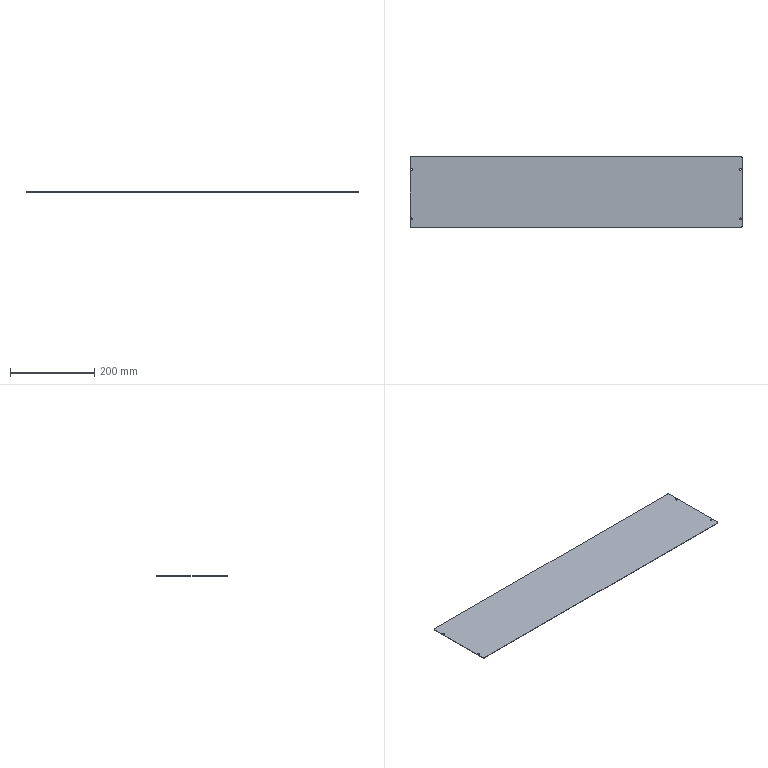Part | SolidWorks | features BaseBody 1 | 1 solid | 18 faces | box 789 x 168 x 1 mm | volume 132481 mm3 | cylinder 12 | plane 6 | commonest cylinder face diameters 4.5 x8 6 x4
STEP:
#1=CARTESIAN_POINT('',(388.25,54.,-1.));
#2=VERTEX_POINT('',#1);
#3=CARTESIAN_POINT('',(392.75,54.,-1.));
#4=VERTEX_POINT('',#3);
#5=CARTESIAN_POINT('',(390.5,54.,-1.));
#6=DIRECTION('',(0.,0.,1.));
#7=DIRECTION('',(1.,0.,0.));
#8=AXIS2_PLACEMENT_3D('',#5,#6,#7);
#9=CIRCLE('',#8,2.25);
#10=EDGE_CURVE('',#2,#4,#9,.T.);
#11=ORIENTED_EDGE('',*,*,#10,.F.);
#12=CARTESIAN_POINT('',(388.25,54.,0.));
#13=VERTEX_POINT('',#12);
#14=CARTESIAN_POINT('',(388.25,54.,-1.));
#15=DIRECTION('',(0.,0.,1.));
#16=VECTOR('',#15,1000.);
#17=LINE('',#14,#16);
#18=EDGE_CURVE('',#2,#13,#17,.T.);
#19=ORIENTED_EDGE('',*,*,#18,.T.);
#20=CARTESIAN_POINT('',(392.75,54.,0.));
#21=VERTEX_POINT('',#20);
#22=CARTESIAN_POINT('',(390.5,54.,0.));
#23=DIRECTION('',(0.,0.,1.));
#24=DIRECTION('',(1.,0.,0.));
#25=AXIS2_PLACEMENT_3D('',#22,#23,#24);
#26=CIRCLE('',#25,2.25);
#27=EDGE_CURVE('',#13,#21,#26,.T.);
#28=ORIENTED_EDGE('',*,*,#27,.T.);
#29=CARTESIAN_POINT('',(392.75,54.,-1.));
#30=DIRECTION('',(0.,0.,1.));
#31=VECTOR('',#30,1000.);
#32=LINE('',#29,#31);
#33=EDGE_CURVE('',#4,#21,#32,.T.);
#34=ORIENTED_EDGE('',*,*,#33,.F.);
#35=EDGE_LOOP('',(#11,#19,#28,#34));
#36=FACE_OUTER_BOUND('',#35,.T.);
#37=CARTESIAN_POINT('',(390.5,54.,-1.));
#38=DIRECTION('',(0.,0.,1.));
#39=DIRECTION('',(1.,0.,0.));
#40=AXIS2_PLACEMENT_3D('',#37,#38,#39);
#41=CYLINDRICAL_SURFACE('',#40,2.25);
#42=ADVANCED_FACE('',(#36),#41,.F.);
#43=CARTESIAN_POINT('',(388.25,-64.,-1.));
#44=VERTEX_POINT('',#43);
#45=CARTESIAN_POINT('',(392.75,-64.,-1.));
#46=VERTEX_POINT('',#45);
#47=CARTESIAN_POINT('',(390.5,-64.,-1.));
#48=DIRECTION('',(0.,0.,1.));
#49=DIRECTION('',(1.,0.,0.));
#50=AXIS2_PLACEMENT_3D('',#47,#48,#49);
#51=CIRCLE('',#50,2.25);
#52=EDGE_CURVE('',#44,#46,#51,.T.);
#53=ORIENTED_EDGE('',*,*,#52,.F.);
#54=CARTESIAN_POINT('',(388.25,-64.,0.));
#55=VERTEX_POINT('',#54);
#56=CARTESIAN_POINT('',(388.25,-64.,-1.));
#57=DIRECTION('',(0.,0.,1.));
#58=VECTOR('',#57,1000.);
#59=LINE('',#56,#58);
#60=EDGE_CURVE('',#44,#55,#59,.T.);
#61=ORIENTED_EDGE('',*,*,#60,.T.);
#62=CARTESIAN_POINT('',(392.75,-64.,0.));
#63=VERTEX_POINT('',#62);
#64=CARTESIAN_POINT('',(390.5,-64.,0.));
#65=DIRECTION('',(0.,0.,1.));
#66=DIRECTION('',(1.,0.,0.));
#67=AXIS2_PLACEMENT_3D('',#64,#65,#66);
#68=CIRCLE('',#67,2.25);
#69=EDGE_CURVE('',#55,#63,#68,.T.);
#70=ORIENTED_EDGE('',*,*,#69,.T.);
#71=CARTESIAN_POINT('',(392.75,-64.,-1.));
#72=DIRECTION('',(0.,0.,1.));
#73=VECTOR('',#72,1000.);
#74=LINE('',#71,#73);
#75=EDGE_CURVE('',#46,#63,#74,.T.);
#76=ORIENTED_EDGE('',*,*,#75,.F.);
#77=EDGE_LOOP('',(#53,#61,#70,#76));
#78=FACE_OUTER_BOUND('',#77,.T.);
#79=CARTESIAN_POINT('',(390.5,-64.,-1.));
#80=DIRECTION('',(0.,0.,1.));
#81=DIRECTION('',(1.,0.,0.));
#82=AXIS2_PLACEMENT_3D('',#79,#80,#81);
#83=CYLINDRICAL_SURFACE('',#82,2.25);
#84=ADVANCED_FACE('',(#78),#83,.F.);
#85=CARTESIAN_POINT('',(-392.75,-64.,-1.));
#86=VERTEX_POINT('',#85);
#87=CARTESIAN_POINT('',(-388.25,-64.,-1.));
#88=VERTEX_POINT('',#87);
#89=CARTESIAN_POINT('',(-390.5,-64.,-1.));
#90=DIRECTION('',(0.,0.,1.));
#91=DIRECTION('',(1.,0.,0.));
#92=AXIS2_PLACEMENT_3D('',#89,#90,#91);
#93=CIRCLE('',#92,2.25);
#94=EDGE_CURVE('',#86,#88,#93,.T.);
#95=ORIENTED_EDGE('',*,*,#94,.F.);
#96=CARTESIAN_POINT('',(-392.75,-64.,0.));
#97=VERTEX_POINT('',#96);
#98=CARTESIAN_POINT('',(-392.75,-64.,-1.));
#99=DIRECTION('',(0.,0.,1.));
#100=VECTOR('',#99,1000.);
#101=LINE('',#98,#100);
#102=EDGE_CURVE('',#86,#97,#101,.T.);
#103=ORIENTED_EDGE('',*,*,#102,.T.);
#104=CARTESIAN_POINT('',(-388.25,-64.,0.));
#105=VERTEX_POINT('',#104);
#106=CARTESIAN_POINT('',(-390.5,-64.,0.));
#107=DIRECTION('',(0.,0.,1.));
#108=DIRECTION('',(1.,0.,0.));
#109=AXIS2_PLACEMENT_3D('',#106,#107,#108);
#110=CIRCLE('',#109,2.25);
#111=EDGE_CURVE('',#97,#105,#110,.T.);
#112=ORIENTED_EDGE('',*,*,#111,.T.);
#113=CARTESIAN_POINT('',(-388.25,-64.,-1.));
#114=DIRECTION('',(0.,0.,1.));
#115=VECTOR('',#114,1000.);
#116=LINE('',#113,#115);
#117=EDGE_CURVE('',#88,#105,#116,.T.);
#118=ORIENTED_EDGE('',*,*,#117,.F.);
#119=EDGE_LOOP('',(#95,#103,#112,#118));
#120=FACE_OUTER_BOUND('',#119,.T.);
#121=CARTESIAN_POINT('',(-390.5,-64.,-1.));
#122=DIRECTION('',(0.,0.,1.));
#123=DIRECTION('',(1.,0.,0.));
#124=AXIS2_PLACEMENT_3D('',#121,#122,#123);
#125=CYLINDRICAL_SURFACE('',#124,2.25);
#126=ADVANCED_FACE('',(#120),#125,.F.);
#127=CARTESIAN_POINT('',(-392.75,54.,-1.));
#128=VERTEX_POINT('',#127);
#129=CARTESIAN_POINT('',(-388.25,54.,-1.));
#130=VERTEX_POINT('',#129);
#131=CARTESIAN_POINT('',(-390.5,54.,-1.));
#132=DIRECTION('',(0.,0.,1.));
#133=DIRECTION('',(1.,0.,0.));
#134=AXIS2_PLACEMENT_3D('',#131,#132,#133);
#135=CIRCLE('',#134,2.25);
#136=EDGE_CURVE('',#128,#130,#135,.T.);
#137=ORIENTED_EDGE('',*,*,#136,.F.);
#138=CARTESIAN_POINT('',(-392.75,54.,0.));
#139=VERTEX_POINT('',#138);
#140=CARTESIAN_POINT('',(-392.75,54.,-1.));
#141=DIRECTION('',(0.,0.,1.));
#142=VECTOR('',#141,1000.);
#143=LINE('',#140,#142);
#144=EDGE_CURVE('',#128,#139,#143,.T.);
#145=ORIENTED_EDGE('',*,*,#144,.T.);
#146=CARTESIAN_POINT('',(-388.25,54.,0.));
#147=VERTEX_POINT('',#146);
#148=CARTESIAN_POINT('',(-390.5,54.,0.));
#149=DIRECTION('',(0.,0.,1.));
#150=DIRECTION('',(1.,0.,0.));
#151=AXIS2_PLACEMENT_3D('',#148,#149,#150);
#152=CIRCLE('',#151,2.25);
#153=EDGE_CURVE('',#139,#147,#152,.T.);
#154=ORIENTED_EDGE('',*,*,#153,.T.);
#155=CARTESIAN_POINT('',(-388.25,54.,-1.));
#156=DIRECTION('',(0.,0.,1.));
#157=VECTOR('',#156,1000.);
#158=LINE('',#155,#157);
#159=EDGE_CURVE('',#130,#147,#158,.T.);
#160=ORIENTED_EDGE('',*,*,#159,.F.);
#161=EDGE_LOOP('',(#137,#145,#154,#160));
#162=FACE_OUTER_BOUND('',#161,.T.);
#163=CARTESIAN_POINT('',(-390.5,54.,-1.));
#164=DIRECTION('',(0.,0.,1.));
#165=DIRECTION('',(1.,0.,0.));
#166=AXIS2_PLACEMENT_3D('',#163,#164,#165);
#167=CYLINDRICAL_SURFACE('',#166,2.25);
#168=ADVANCED_FACE('',(#162),#167,.F.);
#169=CARTESIAN_POINT('',(-390.5,54.,-1.));
#170=DIRECTION('',(0.,0.,1.));
#171=DIRECTION('',(1.,0.,0.));
#172=AXIS2_PLACEMENT_3D('',#169,#170,#171);
#173=CIRCLE('',#172,2.25);
#174=EDGE_CURVE('',#130,#128,#173,.T.);
#175=ORIENTED_EDGE('',*,*,#174,.T.);
#176=ORIENTED_EDGE('',*,*,#136,.T.);
#177=EDGE_LOOP('',(#175,#176));
#178=FACE_BOUND('',#177,.T.);
#179=CARTESIAN_POINT('',(-390.5,-64.,-1.));
#180=DIRECTION('',(0.,0.,1.));
#181=DIRECTION('',(1.,0.,0.));
#182=AXIS2_PLACEMENT_3D('',#179,#180,#181);
#183=CIRCLE('',#182,2.25);
#184=EDGE_CURVE('',#88,#86,#183,.T.);
#185=ORIENTED_EDGE('',*,*,#184,.T.);
#186=ORIENTED_EDGE('',*,*,#94,.T.);
#187=EDGE_LOOP('',(#185,#186));
#188=FACE_BOUND('',#187,.T.);
#189=CARTESIAN_POINT('',(390.5,-64.,-1.));
#190=DIRECTION('',(0.,0.,1.));
#191=DIRECTION('',(1.,0.,0.));
#192=AXIS2_PLACEMENT_3D('',#189,#190,#191);
#193=CIRCLE('',#192,2.25);
#194=EDGE_CURVE('',#46,#44,#193,.T.);
#195=ORIENTED_EDGE('',*,*,#194,.T.);
#196=ORIENTED_EDGE('',*,*,#52,.T.);
#197=EDGE_LOOP('',(#195,#196));
#198=FACE_BOUND('',#197,.T.);
#199=CARTESIAN_POINT('',(390.5,54.,-1.));
#200=DIRECTION('',(0.,0.,1.));
#201=DIRECTION('',(1.,0.,0.));
#202=AXIS2_PLACEMENT_3D('',#199,#200,#201);
#203=CIRCLE('',#202,2.25);
#204=EDGE_CURVE('',#4,#2,#203,.T.);
#205=ORIENTED_EDGE('',*,*,#204,.T.);
#206=ORIENTED_EDGE('',*,*,#10,.T.);
#207=EDGE_LOOP('',(#205,#206));
#208=FACE_BOUND('',#207,.T.);
#209=CARTESIAN_POINT('',(391.5,84.,-1.));
#210=VERTEX_POINT('',#209);
#211=CARTESIAN_POINT('',(-391.5,84.,-1.));
#212=VERTEX_POINT('',#211);
#213=CARTESIAN_POINT('',(-394.5,84.,-1.));
#214=DIRECTION('',(-1.,0.,0.));
#215=VECTOR('',#214,1000.);
#216=LINE('',#213,#215);
#217=EDGE_CURVE('',#210,#212,#216,.T.);
#218=ORIENTED_EDGE('',*,*,#217,.F.);
#219=CARTESIAN_POINT('',(394.5,81.,-1.));
#220=VERTEX_POINT('',#219);
#221=CARTESIAN_POINT('',(391.5,81.,-1.));
#222=DIRECTION('',(0.,0.,1.));
#223=DIRECTION('',(1.,0.,0.));
#224=AXIS2_PLACEMENT_3D('',#221,#222,#223);
#225=CIRCLE('',#224,3.);
#226=EDGE_CURVE('',#220,#210,#225,.T.);
#227=ORIENTED_EDGE('',*,*,#226,.F.);
#228=CARTESIAN_POINT('',(394.5,-81.,-1.));
#229=VERTEX_POINT('',#228);
#230=CARTESIAN_POINT('',(394.5,-84.,-1.));
#231=DIRECTION('',(0.,1.,0.));
#232=VECTOR('',#231,1000.);
#233=LINE('',#230,#232);
#234=EDGE_CURVE('',#229,#220,#233,.T.);
#235=ORIENTED_EDGE('',*,*,#234,.F.);
#236=CARTESIAN_POINT('',(391.5,-84.,-1.));
#237=VERTEX_POINT('',#236);
#238=CARTESIAN_POINT('',(391.5,-81.,-1.));
#239=DIRECTION('',(0.,0.,1.));
#240=DIRECTION('',(1.,0.,0.));
#241=AXIS2_PLACEMENT_3D('',#238,#239,#240);
#242=CIRCLE('',#241,3.);
#243=EDGE_CURVE('',#237,#229,#242,.T.);
#244=ORIENTED_EDGE('',*,*,#243,.F.);
#245=CARTESIAN_POINT('',(-391.5,-84.,-1.));
#246=VERTEX_POINT('',#245);
#247=CARTESIAN_POINT('',(-394.5,-84.,-1.));
#248=DIRECTION('',(1.,0.,0.));
#249=VECTOR('',#248,1000.);
#250=LINE('',#247,#249);
#251=EDGE_CURVE('',#246,#237,#250,.T.);
#252=ORIENTED_EDGE('',*,*,#251,.F.);
#253=CARTESIAN_POINT('',(-394.5,-81.,-1.));
#254=VERTEX_POINT('',#253);
#255=CARTESIAN_POINT('',(-391.5,-81.,-1.));
#256=DIRECTION('',(0.,0.,1.));
#257=DIRECTION('',(1.,0.,0.));
#258=AXIS2_PLACEMENT_3D('',#255,#256,#257);
#259=CIRCLE('',#258,3.);
#260=EDGE_CURVE('',#254,#246,#259,.T.);
#261=ORIENTED_EDGE('',*,*,#260,.F.);
#262=CARTESIAN_POINT('',(-394.5,81.,-1.));
#263=VERTEX_POINT('',#262);
#264=CARTESIAN_POINT('',(-394.5,-84.,-1.));
#265=DIRECTION('',(0.,-1.,0.));
#266=VECTOR('',#265,1000.);
#267=LINE('',#264,#266);
#268=EDGE_CURVE('',#263,#254,#267,.T.);
#269=ORIENTED_EDGE('',*,*,#268,.F.);
#270=CARTESIAN_POINT('',(-391.5,81.,-1.));
#271=DIRECTION('',(0.,0.,1.));
#272=DIRECTION('',(1.,0.,0.));
#273=AXIS2_PLACEMENT_3D('',#270,#271,#272);
#274=CIRCLE('',#273,3.);
#275=EDGE_CURVE('',#212,#263,#274,.T.);
#276=ORIENTED_EDGE('',*,*,#275,.F.);
#277=EDGE_LOOP('',(#218,#227,#235,#244,#252,#261,#269,#276));
#278=FACE_OUTER_BOUND('',#277,.T.);
#279=CARTESIAN_POINT('',(0.,0.,-1.));
#280=DIRECTION('',(0.,0.,-1.));
#281=DIRECTION('',(0.,-1.,0.));
#282=AXIS2_PLACEMENT_3D('',#279,#280,#281);
#283=PLANE('',#282);
#284=ADVANCED_FACE('',(#178,#188,#198,#208,#278),#283,.T.);
#285=CARTESIAN_POINT('',(-391.5,-84.,0.));
#286=VERTEX_POINT('',#285);
#287=CARTESIAN_POINT('',(-394.5,-81.,0.));
#288=VERTEX_POINT('',#287);
#289=CARTESIAN_POINT('',(-391.5,-81.,0.));
#290=DIRECTION('',(0.,0.,-1.));
#291=DIRECTION('',(1.,0.,0.));
#292=AXIS2_PLACEMENT_3D('',#289,#290,#291);
#293=CIRCLE('',#292,3.);
#294=EDGE_CURVE('',#286,#288,#293,.T.);
#295=ORIENTED_EDGE('',*,*,#294,.T.);
#296=CARTESIAN_POINT('',(-394.5,-81.,-1.));
#297=DIRECTION('',(0.,0.,1.));
#298=VECTOR('',#297,1000.);
#299=LINE('',#296,#298);
#300=EDGE_CURVE('',#254,#288,#299,.T.);
#301=ORIENTED_EDGE('',*,*,#300,.F.);
#302=ORIENTED_EDGE('',*,*,#260,.T.);
#303=CARTESIAN_POINT('',(-391.5,-84.,-1.));
#304=DIRECTION('',(0.,0.,-1.));
#305=VECTOR('',#304,1000.);
#306=LINE('',#303,#305);
#307=EDGE_CURVE('',#286,#246,#306,.T.);
#308=ORIENTED_EDGE('',*,*,#307,.F.);
#309=EDGE_LOOP('',(#295,#301,#302,#308));
#310=FACE_OUTER_BOUND('',#309,.T.);
#311=CARTESIAN_POINT('',(-391.5,-81.,-1.));
#312=DIRECTION('',(0.,0.,1.));
#313=DIRECTION('',(1.,0.,0.));
#314=AXIS2_PLACEMENT_3D('',#311,#312,#313);
#315=CYLINDRICAL_SURFACE('',#314,3.);
#316=ADVANCED_FACE('',(#310),#315,.T.);
#317=CARTESIAN_POINT('',(-394.5,81.,0.));
#318=VERTEX_POINT('',#317);
#319=CARTESIAN_POINT('',(-394.5,0.,0.));
#320=DIRECTION('',(0.,1.,0.));
#321=VECTOR('',#320,1000.);
#322=LINE('',#319,#321);
#323=EDGE_CURVE('',#288,#318,#322,.T.);
#324=ORIENTED_EDGE('',*,*,#323,.T.);
#325=CARTESIAN_POINT('',(-394.5,81.,-1.));
#326=DIRECTION('',(0.,0.,1.));
#327=VECTOR('',#326,1000.);
#328=LINE('',#325,#327);
#329=EDGE_CURVE('',#263,#318,#328,.T.);
#330=ORIENTED_EDGE('',*,*,#329,.F.);
#331=ORIENTED_EDGE('',*,*,#268,.T.);
#332=ORIENTED_EDGE('',*,*,#300,.T.);
#333=EDGE_LOOP('',(#324,#330,#331,#332));
#334=FACE_OUTER_BOUND('',#333,.T.);
#335=CARTESIAN_POINT('',(-394.5,-84.,-1.));
#336=DIRECTION('',(-1.,0.,0.));
#337=DIRECTION('',(0.,0.,1.));
#338=AXIS2_PLACEMENT_3D('',#335,#336,#337);
#339=PLANE('',#338);
#340=ADVANCED_FACE('',(#334),#339,.T.);
#341=CARTESIAN_POINT('',(-391.5,84.,0.));
#342=VERTEX_POINT('',#341);
#343=CARTESIAN_POINT('',(-391.5,81.,0.));
#344=DIRECTION('',(0.,0.,-1.));
#345=DIRECTION('',(1.,0.,0.));
#346=AXIS2_PLACEMENT_3D('',#343,#344,#345);
#347=CIRCLE('',#346,3.);
#348=EDGE_CURVE('',#318,#342,#347,.T.);
#349=ORIENTED_EDGE('',*,*,#348,.T.);
#350=CARTESIAN_POINT('',(-391.5,84.,-1.));
#351=DIRECTION('',(0.,0.,1.));
#352=VECTOR('',#351,1000.);
#353=LINE('',#350,#352);
#354=EDGE_CURVE('',#212,#342,#353,.T.);
#355=ORIENTED_EDGE('',*,*,#354,.F.);
#356=ORIENTED_EDGE('',*,*,#275,.T.);
#357=ORIENTED_EDGE('',*,*,#329,.T.);
#358=EDGE_LOOP('',(#349,#355,#356,#357));
#359=FACE_OUTER_BOUND('',#358,.T.);
#360=CARTESIAN_POINT('',(-391.5,81.,-1.));
#361=DIRECTION('',(0.,0.,1.));
#362=DIRECTION('',(1.,0.,0.));
#363=AXIS2_PLACEMENT_3D('',#360,#361,#362);
#364=CYLINDRICAL_SURFACE('',#363,3.);
#365=ADVANCED_FACE('',(#359),#364,.T.);
#366=CARTESIAN_POINT('',(391.5,84.,0.));
#367=VERTEX_POINT('',#366);
#368=CARTESIAN_POINT('',(0.,84.,0.));
#369=DIRECTION('',(1.,0.,0.));
#370=VECTOR('',#369,1000.);
#371=LINE('',#368,#370);
#372=EDGE_CURVE('',#342,#367,#371,.T.);
#373=ORIENTED_EDGE('',*,*,#372,.T.);
#374=CARTESIAN_POINT('',(391.5,84.,-1.));
#375=DIRECTION('',(0.,0.,1.));
#376=VECTOR('',#375,1000.);
#377=LINE('',#374,#376);
#378=EDGE_CURVE('',#210,#367,#377,.T.);
#379=ORIENTED_EDGE('',*,*,#378,.F.);
#380=ORIENTED_EDGE('',*,*,#217,.T.);
#381=ORIENTED_EDGE('',*,*,#354,.T.);
#382=EDGE_LOOP('',(#373,#379,#380,#381));
#383=FACE_OUTER_BOUND('',#382,.T.);
#384=CARTESIAN_POINT('',(-394.5,84.,-1.));
#385=DIRECTION('',(0.,1.,0.));
#386=DIRECTION('',(1.,0.,0.));
#387=AXIS2_PLACEMENT_3D('',#384,#385,#386);
#388=PLANE('',#387);
#389=ADVANCED_FACE('',(#383),#388,.T.);
#390=CARTESIAN_POINT('',(394.5,81.,0.));
#391=VERTEX_POINT('',#390);
#392=CARTESIAN_POINT('',(391.5,81.,0.));
#393=DIRECTION('',(0.,0.,-1.));
#394=DIRECTION('',(1.,0.,0.));
#395=AXIS2_PLACEMENT_3D('',#392,#393,#394);
#396=CIRCLE('',#395,3.);
#397=EDGE_CURVE('',#367,#391,#396,.T.);
#398=ORIENTED_EDGE('',*,*,#397,.T.);
#399=CARTESIAN_POINT('',(394.5,81.,-1.));
#400=DIRECTION('',(0.,0.,1.));
#401=VECTOR('',#400,1000.);
#402=LINE('',#399,#401);
#403=EDGE_CURVE('',#220,#391,#402,.T.);
#404=ORIENTED_EDGE('',*,*,#403,.F.);
#405=ORIENTED_EDGE('',*,*,#226,.T.);
#406=ORIENTED_EDGE('',*,*,#378,.T.);
#407=EDGE_LOOP('',(#398,#404,#405,#406));
#408=FACE_OUTER_BOUND('',#407,.T.);
#409=CARTESIAN_POINT('',(391.5,81.,-1.));
#410=DIRECTION('',(0.,0.,1.));
#411=DIRECTION('',(1.,0.,0.));
#412=AXIS2_PLACEMENT_3D('',#409,#410,#411);
#413=CYLINDRICAL_SURFACE('',#412,3.);
#414=ADVANCED_FACE('',(#408),#413,.T.);
#415=ORIENTED_EDGE('',*,*,#234,.T.);
#416=ORIENTED_EDGE('',*,*,#403,.T.);
#417=CARTESIAN_POINT('',(394.5,-81.,0.));
#418=VERTEX_POINT('',#417);
#419=CARTESIAN_POINT('',(394.5,0.,0.));
#420=DIRECTION('',(0.,-1.,0.));
#421=VECTOR('',#420,1000.);
#422=LINE('',#419,#421);
#423=EDGE_CURVE('',#391,#418,#422,.T.);
#424=ORIENTED_EDGE('',*,*,#423,.T.);
#425=CARTESIAN_POINT('',(394.5,-81.,-1.));
#426=DIRECTION('',(0.,0.,1.));
#427=VECTOR('',#426,1000.);
#428=LINE('',#425,#427);
#429=EDGE_CURVE('',#229,#418,#428,.T.);
#430=ORIENTED_EDGE('',*,*,#429,.F.);
#431=EDGE_LOOP('',(#415,#416,#424,#430));
#432=FACE_OUTER_BOUND('',#431,.T.);
#433=CARTESIAN_POINT('',(394.5,-84.,-1.));
#434=DIRECTION('',(1.,0.,0.));
#435=DIRECTION('',(0.,1.,0.));
#436=AXIS2_PLACEMENT_3D('',#433,#434,#435);
#437=PLANE('',#436);
#438=ADVANCED_FACE('',(#432),#437,.T.);
#439=CARTESIAN_POINT('',(391.5,-84.,0.));
#440=VERTEX_POINT('',#439);
#441=CARTESIAN_POINT('',(391.5,-81.,0.));
#442=DIRECTION('',(0.,0.,-1.));
#443=DIRECTION('',(1.,0.,0.));
#444=AXIS2_PLACEMENT_3D('',#441,#442,#443);
#445=CIRCLE('',#444,3.);
#446=EDGE_CURVE('',#418,#440,#445,.T.);
#447=ORIENTED_EDGE('',*,*,#446,.T.);
#448=CARTESIAN_POINT('',(391.5,-84.,-1.));
#449=DIRECTION('',(0.,0.,1.));
#450=VECTOR('',#449,1000.);
#451=LINE('',#448,#450);
#452=EDGE_CURVE('',#237,#440,#451,.T.);
#453=ORIENTED_EDGE('',*,*,#452,.F.);
#454=ORIENTED_EDGE('',*,*,#243,.T.);
#455=ORIENTED_EDGE('',*,*,#429,.T.);
#456=EDGE_LOOP('',(#447,#453,#454,#455));
#457=FACE_OUTER_BOUND('',#456,.T.);
#458=CARTESIAN_POINT('',(391.5,-81.,-1.));
#459=DIRECTION('',(0.,0.,1.));
#460=DIRECTION('',(1.,0.,0.));
#461=AXIS2_PLACEMENT_3D('',#458,#459,#460);
#462=CYLINDRICAL_SURFACE('',#461,3.);
#463=ADVANCED_FACE('',(#457),#462,.T.);
#464=CARTESIAN_POINT('',(0.,-84.,0.));
#465=DIRECTION('',(-1.,0.,0.));
#466=VECTOR('',#465,1000.);
#467=LINE('',#464,#466);
#468=EDGE_CURVE('',#440,#286,#467,.T.);
#469=ORIENTED_EDGE('',*,*,#468,.T.);
#470=ORIENTED_EDGE('',*,*,#307,.T.);
#471=ORIENTED_EDGE('',*,*,#251,.T.);
#472=ORIENTED_EDGE('',*,*,#452,.T.);
#473=EDGE_LOOP('',(#469,#470,#471,#472));
#474=FACE_OUTER_BOUND('',#473,.T.);
#475=CARTESIAN_POINT('',(-394.5,-84.,-1.));
#476=DIRECTION('',(0.,-1.,0.));
#477=DIRECTION('',(0.,0.,-1.));
#478=AXIS2_PLACEMENT_3D('',#475,#476,#477);
#479=PLANE('',#478);
#480=ADVANCED_FACE('',(#474),#479,.T.);
#481=CARTESIAN_POINT('',(-390.5,54.,0.));
#482=DIRECTION('',(0.,0.,1.));
#483=DIRECTION('',(1.,0.,0.));
#484=AXIS2_PLACEMENT_3D('',#481,#482,#483);
#485=CIRCLE('',#484,2.25);
#486=EDGE_CURVE('',#147,#139,#485,.T.);
#487=ORIENTED_EDGE('',*,*,#486,.F.);
#488=ORIENTED_EDGE('',*,*,#153,.F.);
#489=EDGE_LOOP('',(#487,#488));
#490=FACE_BOUND('',#489,.T.);
#491=CARTESIAN_POINT('',(-390.5,-64.,0.));
#492=DIRECTION('',(0.,0.,1.));
#493=DIRECTION('',(1.,0.,0.));
#494=AXIS2_PLACEMENT_3D('',#491,#492,#493);
#495=CIRCLE('',#494,2.25);
#496=EDGE_CURVE('',#105,#97,#495,.T.);
#497=ORIENTED_EDGE('',*,*,#496,.F.);
#498=ORIENTED_EDGE('',*,*,#111,.F.);
#499=EDGE_LOOP('',(#497,#498));
#500=FACE_BOUND('',#499,.T.);
#501=CARTESIAN_POINT('',(390.5,-64.,0.));
#502=DIRECTION('',(0.,0.,1.));
#503=DIRECTION('',(1.,0.,0.));
#504=AXIS2_PLACEMENT_3D('',#501,#502,#503);
#505=CIRCLE('',#504,2.25);
#506=EDGE_CURVE('',#63,#55,#505,.T.);
#507=ORIENTED_EDGE('',*,*,#506,.F.);
#508=ORIENTED_EDGE('',*,*,#69,.F.);
#509=EDGE_LOOP('',(#507,#508));
#510=FACE_BOUND('',#509,.T.);
#511=CARTESIAN_POINT('',(390.5,54.,0.));
#512=DIRECTION('',(0.,0.,1.));
#513=DIRECTION('',(1.,0.,0.));
#514=AXIS2_PLACEMENT_3D('',#511,#512,#513);
#515=CIRCLE('',#514,2.25);
#516=EDGE_CURVE('',#21,#13,#515,.T.);
#517=ORIENTED_EDGE('',*,*,#516,.F.);
#518=ORIENTED_EDGE('',*,*,#27,.F.);
#519=EDGE_LOOP('',(#517,#518));
#520=FACE_BOUND('',#519,.T.);
#521=ORIENTED_EDGE('',*,*,#446,.F.);
#522=ORIENTED_EDGE('',*,*,#423,.F.);
#523=ORIENTED_EDGE('',*,*,#397,.F.);
#524=ORIENTED_EDGE('',*,*,#372,.F.);
#525=ORIENTED_EDGE('',*,*,#348,.F.);
#526=ORIENTED_EDGE('',*,*,#323,.F.);
#527=ORIENTED_EDGE('',*,*,#294,.F.);
#528=ORIENTED_EDGE('',*,*,#468,.F.);
#529=EDGE_LOOP('',(#521,#522,#523,#524,#525,#526,#527,#528));
#530=FACE_OUTER_BOUND('',#529,.T.);
#531=CARTESIAN_POINT('',(0.,0.,0.));
#532=DIRECTION('',(0.,0.,-1.));
#533=DIRECTION('',(0.,-1.,0.));
#534=AXIS2_PLACEMENT_3D('',#531,#532,#533);
#535=PLANE('',#534);
#536=ADVANCED_FACE('',(#490,#500,#510,#520,#530),#535,.F.);
#537=ORIENTED_EDGE('',*,*,#144,.F.);
#538=ORIENTED_EDGE('',*,*,#174,.F.);
#539=ORIENTED_EDGE('',*,*,#159,.T.);
#540=ORIENTED_EDGE('',*,*,#486,.T.);
#541=EDGE_LOOP('',(#537,#538,#539,#540));
#542=FACE_OUTER_BOUND('',#541,.T.);
#543=CARTESIAN_POINT('',(-390.5,54.,-1.));
#544=DIRECTION('',(0.,0.,1.));
#545=DIRECTION('',(1.,0.,0.));
#546=AXIS2_PLACEMENT_3D('',#543,#544,#545);
#547=CYLINDRICAL_SURFACE('',#546,2.25);
#548=ADVANCED_FACE('',(#542),#547,.F.);
#549=ORIENTED_EDGE('',*,*,#102,.F.);
#550=ORIENTED_EDGE('',*,*,#184,.F.);
#551=ORIENTED_EDGE('',*,*,#117,.T.);
#552=ORIENTED_EDGE('',*,*,#496,.T.);
#553=EDGE_LOOP('',(#549,#550,#551,#552));
#554=FACE_OUTER_BOUND('',#553,.T.);
#555=CARTESIAN_POINT('',(-390.5,-64.,-1.));
#556=DIRECTION('',(0.,0.,1.));
#557=DIRECTION('',(1.,0.,0.));
#558=AXIS2_PLACEMENT_3D('',#555,#556,#557);
#559=CYLINDRICAL_SURFACE('',#558,2.25);
#560=ADVANCED_FACE('',(#554),#559,.F.);
#561=ORIENTED_EDGE('',*,*,#60,.F.);
#562=ORIENTED_EDGE('',*,*,#194,.F.);
#563=ORIENTED_EDGE('',*,*,#75,.T.);
#564=ORIENTED_EDGE('',*,*,#506,.T.);
#565=EDGE_LOOP('',(#561,#562,#563,#564));
#566=FACE_OUTER_BOUND('',#565,.T.);
#567=CARTESIAN_POINT('',(390.5,-64.,-1.));
#568=DIRECTION('',(0.,0.,1.));
#569=DIRECTION('',(1.,0.,0.));
#570=AXIS2_PLACEMENT_3D('',#567,#568,#569);
#571=CYLINDRICAL_SURFACE('',#570,2.25);
#572=ADVANCED_FACE('',(#566),#571,.F.);
#573=ORIENTED_EDGE('',*,*,#18,.F.);
#574=ORIENTED_EDGE('',*,*,#204,.F.);
#575=ORIENTED_EDGE('',*,*,#33,.T.);
#576=ORIENTED_EDGE('',*,*,#516,.T.);
#577=EDGE_LOOP('',(#573,#574,#575,#576));
#578=FACE_OUTER_BOUND('',#577,.T.);
#579=CARTESIAN_POINT('',(390.5,54.,-1.));
#580=DIRECTION('',(0.,0.,1.));
#581=DIRECTION('',(1.,0.,0.));
#582=AXIS2_PLACEMENT_3D('',#579,#580,#581);
#583=CYLINDRICAL_SURFACE('',#582,2.25);
#584=ADVANCED_FACE('',(#578),#583,.F.);
#585=CLOSED_SHELL('',(#42,#84,#126,#168,#284,#316,#340,#365,#389,#414,#438,#463,#480,#536,#548,#560,#572,#584));
#586=MANIFOLD_SOLID_BREP('',#585);
#587=CARTESIAN_POINT('',(0.,0.,0.));
#588=DIRECTION('',(0.,0.,1.));
#589=DIRECTION('',(1.,0.,0.));
#590=AXIS2_PLACEMENT_3D('',#587,#588,#589);
#591=(LENGTH_UNIT()NAMED_UNIT(*)SI_UNIT(.MILLI.,.METRE.));
#592=UNCERTAINTY_MEASURE_WITH_UNIT(LENGTH_MEASURE(0.00001),#591,'','');
#593=(NAMED_UNIT(*)PLANE_ANGLE_UNIT()SI_UNIT($,.RADIAN.));
#594=(NAMED_UNIT(*)SI_UNIT($,.STERADIAN.)SOLID_ANGLE_UNIT());
#595=(GEOMETRIC_REPRESENTATION_CONTEXT(3)GLOBAL_UNCERTAINTY_ASSIGNED_CONTEXT((#592))GLOBAL_UNIT_ASSIGNED_CONTEXT((#591,#593,#594))REPRESENTATION_CONTEXT('',''));
#596=ADVANCED_BREP_SHAPE_REPRESENTATION('',(#586,#590),#595);